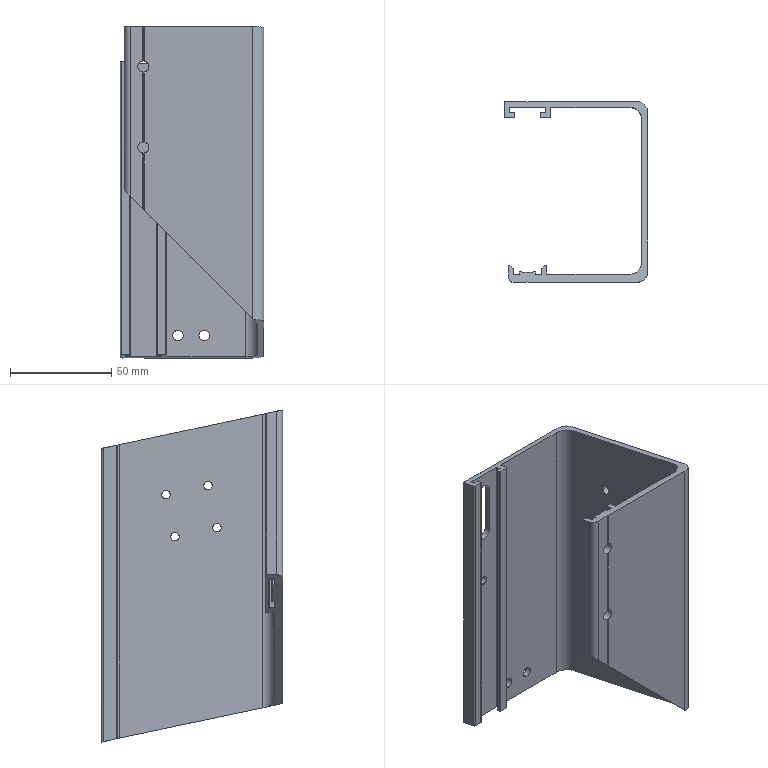Part | STEP file | 31E-01009XJ12 | 1 solid | 87 faces | box 71 x 89.5 x 164.024 mm | volume 105161 mm3 | plane 44 | cylinder 43 | commonest cylinder face diameters 1 x10 4.2 x10 5.2 x4 5.5 x4 8 x4 25.4 x3